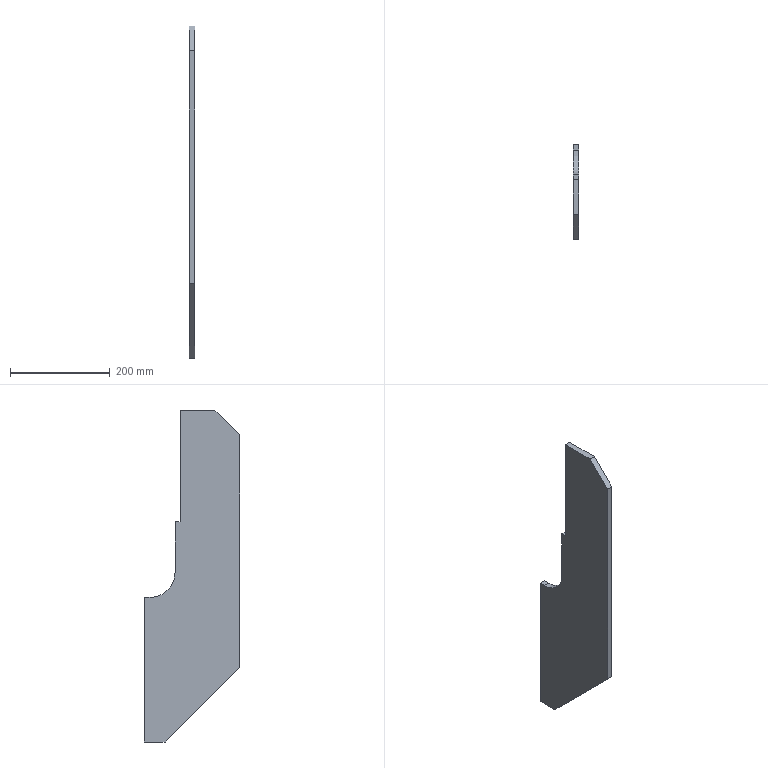Part | STEP file | CENTERING.RIB.1.stp | 1 solid | 37 faces | box 12 x 192 x 666 mm | volume 1081564 mm3 | spline 22 | cylinder 10 | plane 5 | commonest cylinder face diameters 6 x10